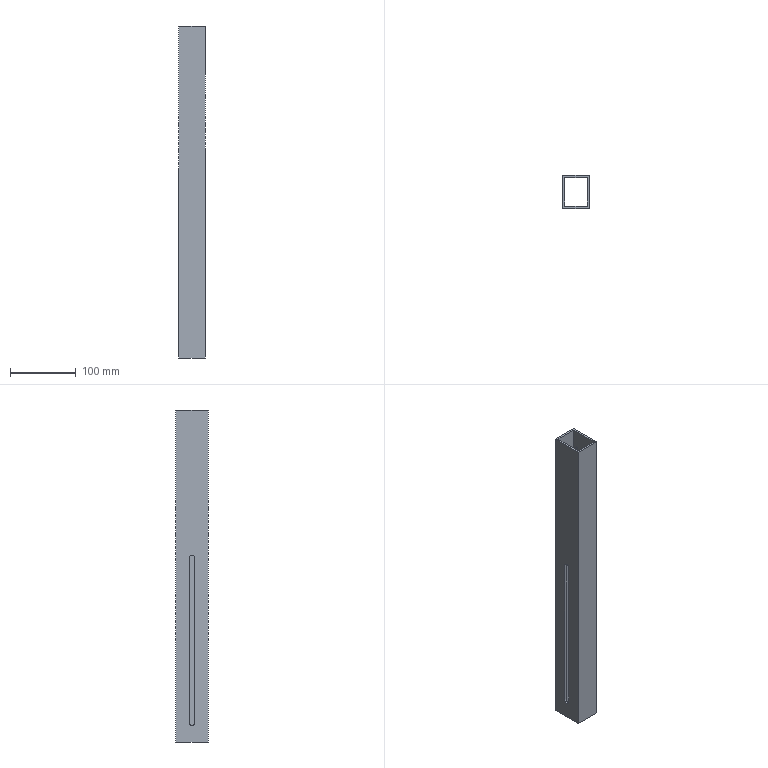Part | SolidWorks | features HoleWzd 4, ExtruThin 1 | 1 solid | 39 faces | box 40 x 50 x 506 mm | volume 247347 mm3 | cylinder 27 | plane 12 | commonest cylinder face diameters 5.5 x16 4.2 x8 9 x3
STEP:
#1=CARTESIAN_POINT('',(-17.,4.5,27.));
#2=VERTEX_POINT('',#1);
#3=CARTESIAN_POINT('',(-17.,0.,31.5));
#4=VERTEX_POINT('',#3);
#5=CARTESIAN_POINT('',(-17.,0.,27.));
#6=DIRECTION('',(1.,0.,0.));
#7=DIRECTION('',(0.,1.,0.));
#8=AXIS2_PLACEMENT_3D('',#5,#6,#7);
#9=CIRCLE('',#8,4.5);
#10=EDGE_CURVE('',#2,#4,#9,.T.);
#11=ORIENTED_EDGE('',*,*,#10,.T.);
#12=CARTESIAN_POINT('',(-20.,0.,31.5));
#13=VERTEX_POINT('',#12);
#14=CARTESIAN_POINT('',(-20.,0.,31.5));
#15=DIRECTION('',(-1.,0.,0.));
#16=VECTOR('',#15,1000.);
#17=LINE('',#14,#16);
#18=EDGE_CURVE('',#4,#13,#17,.T.);
#19=ORIENTED_EDGE('',*,*,#18,.T.);
#20=CARTESIAN_POINT('',(-20.,4.5,27.));
#21=VERTEX_POINT('',#20);
#22=CARTESIAN_POINT('',(-20.,0.,27.));
#23=DIRECTION('',(-1.,0.,0.));
#24=DIRECTION('',(0.,0.,1.));
#25=AXIS2_PLACEMENT_3D('',#22,#23,#24);
#26=CIRCLE('',#25,4.5);
#27=EDGE_CURVE('',#13,#21,#26,.T.);
#28=ORIENTED_EDGE('',*,*,#27,.T.);
#29=CARTESIAN_POINT('',(-16.999,4.5,27.));
#30=DIRECTION('',(1.,0.,0.));
#31=VECTOR('',#30,1000.);
#32=LINE('',#29,#31);
#33=EDGE_CURVE('',#21,#2,#32,.T.);
#34=ORIENTED_EDGE('',*,*,#33,.T.);
#35=EDGE_LOOP('',(#11,#19,#28,#34));
#36=FACE_OUTER_BOUND('',#35,.T.);
#37=CARTESIAN_POINT('',(-20.,0.,27.));
#38=DIRECTION('',(-1.,0.,0.));
#39=DIRECTION('',(0.,0.,1.));
#40=AXIS2_PLACEMENT_3D('',#37,#38,#39);
#41=CYLINDRICAL_SURFACE('',#40,4.5);
#42=ADVANCED_FACE('',(#36),#41,.F.);
#43=CARTESIAN_POINT('',(17.,15.,220.9));
#44=VERTEX_POINT('',#43);
#45=CARTESIAN_POINT('',(17.,15.,225.1));
#46=VERTEX_POINT('',#45);
#47=CARTESIAN_POINT('',(17.,15.,223.));
#48=DIRECTION('',(-1.,0.,0.));
#49=DIRECTION('',(0.,-1.,0.));
#50=AXIS2_PLACEMENT_3D('',#47,#48,#49);
#51=CIRCLE('',#50,2.1);
#52=EDGE_CURVE('',#44,#46,#51,.T.);
#53=ORIENTED_EDGE('',*,*,#52,.T.);
#54=CARTESIAN_POINT('',(20.,15.,225.1));
#55=VERTEX_POINT('',#54);
#56=CARTESIAN_POINT('',(20.,15.,225.1));
#57=DIRECTION('',(1.,0.,0.));
#58=VECTOR('',#57,1000.);
#59=LINE('',#56,#58);
#60=EDGE_CURVE('',#46,#55,#59,.T.);
#61=ORIENTED_EDGE('',*,*,#60,.T.);
#62=CARTESIAN_POINT('',(20.,15.,220.9));
#63=VERTEX_POINT('',#62);
#64=CARTESIAN_POINT('',(20.,15.,223.));
#65=DIRECTION('',(1.,0.,0.));
#66=DIRECTION('',(0.,0.,-1.));
#67=AXIS2_PLACEMENT_3D('',#64,#65,#66);
#68=CIRCLE('',#67,2.1);
#69=EDGE_CURVE('',#55,#63,#68,.T.);
#70=ORIENTED_EDGE('',*,*,#69,.T.);
#71=CARTESIAN_POINT('',(20.,15.,220.9));
#72=DIRECTION('',(1.,0.,0.));
#73=VECTOR('',#72,1000.);
#74=LINE('',#71,#73);
#75=EDGE_CURVE('',#44,#63,#74,.T.);
#76=ORIENTED_EDGE('',*,*,#75,.F.);
#77=EDGE_LOOP('',(#53,#61,#70,#76));
#78=FACE_OUTER_BOUND('',#77,.T.);
#79=CARTESIAN_POINT('',(20.,15.,223.));
#80=DIRECTION('',(1.,0.,0.));
#81=DIRECTION('',(0.,0.,-1.));
#82=AXIS2_PLACEMENT_3D('',#79,#80,#81);
#83=CYLINDRICAL_SURFACE('',#82,2.1);
#84=ADVANCED_FACE('',(#78),#83,.F.);
#85=CARTESIAN_POINT('',(17.,-15.,220.9));
#86=VERTEX_POINT('',#85);
#87=CARTESIAN_POINT('',(17.,-15.,225.1));
#88=VERTEX_POINT('',#87);
#89=CARTESIAN_POINT('',(17.,-15.,223.));
#90=DIRECTION('',(-1.,0.,0.));
#91=DIRECTION('',(0.,-1.,0.));
#92=AXIS2_PLACEMENT_3D('',#89,#90,#91);
#93=CIRCLE('',#92,2.1);
#94=EDGE_CURVE('',#86,#88,#93,.T.);
#95=ORIENTED_EDGE('',*,*,#94,.T.);
#96=CARTESIAN_POINT('',(20.,-15.,225.1));
#97=VERTEX_POINT('',#96);
#98=CARTESIAN_POINT('',(20.,-15.,225.1));
#99=DIRECTION('',(1.,0.,0.));
#100=VECTOR('',#99,1000.);
#101=LINE('',#98,#100);
#102=EDGE_CURVE('',#88,#97,#101,.T.);
#103=ORIENTED_EDGE('',*,*,#102,.T.);
#104=CARTESIAN_POINT('',(20.,-15.,220.9));
#105=VERTEX_POINT('',#104);
#106=CARTESIAN_POINT('',(20.,-15.,223.));
#107=DIRECTION('',(1.,0.,0.));
#108=DIRECTION('',(0.,0.,-1.));
#109=AXIS2_PLACEMENT_3D('',#106,#107,#108);
#110=CIRCLE('',#109,2.1);
#111=EDGE_CURVE('',#97,#105,#110,.T.);
#112=ORIENTED_EDGE('',*,*,#111,.T.);
#113=CARTESIAN_POINT('',(20.,-15.,220.9));
#114=DIRECTION('',(1.,0.,0.));
#115=VECTOR('',#114,1000.);
#116=LINE('',#113,#115);
#117=EDGE_CURVE('',#86,#105,#116,.T.);
#118=ORIENTED_EDGE('',*,*,#117,.F.);
#119=EDGE_LOOP('',(#95,#103,#112,#118));
#120=FACE_OUTER_BOUND('',#119,.T.);
#121=CARTESIAN_POINT('',(20.,-15.,223.));
#122=DIRECTION('',(1.,0.,0.));
#123=DIRECTION('',(0.,0.,-1.));
#124=AXIS2_PLACEMENT_3D('',#121,#122,#123);
#125=CYLINDRICAL_SURFACE('',#124,2.1);
#126=ADVANCED_FACE('',(#120),#125,.F.);
#127=CARTESIAN_POINT('',(17.,-15.,-225.1));
#128=VERTEX_POINT('',#127);
#129=CARTESIAN_POINT('',(17.,-15.,-220.9));
#130=VERTEX_POINT('',#129);
#131=CARTESIAN_POINT('',(17.,-15.,-223.));
#132=DIRECTION('',(-1.,0.,0.));
#133=DIRECTION('',(0.,-1.,0.));
#134=AXIS2_PLACEMENT_3D('',#131,#132,#133);
#135=CIRCLE('',#134,2.1);
#136=EDGE_CURVE('',#128,#130,#135,.T.);
#137=ORIENTED_EDGE('',*,*,#136,.T.);
#138=CARTESIAN_POINT('',(20.,-15.,-220.9));
#139=VERTEX_POINT('',#138);
#140=CARTESIAN_POINT('',(20.,-15.,-220.9));
#141=DIRECTION('',(1.,0.,0.));
#142=VECTOR('',#141,1000.);
#143=LINE('',#140,#142);
#144=EDGE_CURVE('',#130,#139,#143,.T.);
#145=ORIENTED_EDGE('',*,*,#144,.T.);
#146=CARTESIAN_POINT('',(20.,-15.,-225.1));
#147=VERTEX_POINT('',#146);
#148=CARTESIAN_POINT('',(20.,-15.,-223.));
#149=DIRECTION('',(1.,0.,0.));
#150=DIRECTION('',(0.,0.,-1.));
#151=AXIS2_PLACEMENT_3D('',#148,#149,#150);
#152=CIRCLE('',#151,2.1);
#153=EDGE_CURVE('',#139,#147,#152,.T.);
#154=ORIENTED_EDGE('',*,*,#153,.T.);
#155=CARTESIAN_POINT('',(20.,-15.,-225.1));
#156=DIRECTION('',(1.,0.,0.));
#157=VECTOR('',#156,1000.);
#158=LINE('',#155,#157);
#159=EDGE_CURVE('',#128,#147,#158,.T.);
#160=ORIENTED_EDGE('',*,*,#159,.F.);
#161=EDGE_LOOP('',(#137,#145,#154,#160));
#162=FACE_OUTER_BOUND('',#161,.T.);
#163=CARTESIAN_POINT('',(20.,-15.,-223.));
#164=DIRECTION('',(1.,0.,0.));
#165=DIRECTION('',(0.,0.,-1.));
#166=AXIS2_PLACEMENT_3D('',#163,#164,#165);
#167=CYLINDRICAL_SURFACE('',#166,2.1);
#168=ADVANCED_FACE('',(#162),#167,.F.);
#169=CARTESIAN_POINT('',(17.,15.,-225.1));
#170=VERTEX_POINT('',#169);
#171=CARTESIAN_POINT('',(17.,15.,-220.9));
#172=VERTEX_POINT('',#171);
#173=CARTESIAN_POINT('',(17.,15.,-223.));
#174=DIRECTION('',(-1.,0.,0.));
#175=DIRECTION('',(0.,-1.,0.));
#176=AXIS2_PLACEMENT_3D('',#173,#174,#175);
#177=CIRCLE('',#176,2.1);
#178=EDGE_CURVE('',#170,#172,#177,.T.);
#179=ORIENTED_EDGE('',*,*,#178,.T.);
#180=CARTESIAN_POINT('',(20.,15.,-220.9));
#181=VERTEX_POINT('',#180);
#182=CARTESIAN_POINT('',(20.,15.,-220.9));
#183=DIRECTION('',(1.,0.,0.));
#184=VECTOR('',#183,1000.);
#185=LINE('',#182,#184);
#186=EDGE_CURVE('',#172,#181,#185,.T.);
#187=ORIENTED_EDGE('',*,*,#186,.T.);
#188=CARTESIAN_POINT('',(20.,15.,-225.1));
#189=VERTEX_POINT('',#188);
#190=CARTESIAN_POINT('',(20.,15.,-223.));
#191=DIRECTION('',(1.,0.,0.));
#192=DIRECTION('',(0.,0.,-1.));
#193=AXIS2_PLACEMENT_3D('',#190,#191,#192);
#194=CIRCLE('',#193,2.1);
#195=EDGE_CURVE('',#181,#189,#194,.T.);
#196=ORIENTED_EDGE('',*,*,#195,.T.);
#197=CARTESIAN_POINT('',(20.,15.,-225.1));
#198=DIRECTION('',(1.,0.,0.));
#199=VECTOR('',#198,1000.);
#200=LINE('',#197,#199);
#201=EDGE_CURVE('',#170,#189,#200,.T.);
#202=ORIENTED_EDGE('',*,*,#201,.F.);
#203=EDGE_LOOP('',(#179,#187,#196,#202));
#204=FACE_OUTER_BOUND('',#203,.T.);
#205=CARTESIAN_POINT('',(20.,15.,-223.));
#206=DIRECTION('',(1.,0.,0.));
#207=DIRECTION('',(0.,0.,-1.));
#208=AXIS2_PLACEMENT_3D('',#205,#206,#207);
#209=CYLINDRICAL_SURFACE('',#208,2.1);
#210=ADVANCED_FACE('',(#204),#209,.F.);
#211=CARTESIAN_POINT('',(17.,16.,179.5));
#212=VERTEX_POINT('',#211);
#213=CARTESIAN_POINT('',(17.,16.,185.));
#214=VERTEX_POINT('',#213);
#215=CARTESIAN_POINT('',(17.,16.,182.25));
#216=DIRECTION('',(-1.,0.,0.));
#217=DIRECTION('',(0.,-1.,0.));
#218=AXIS2_PLACEMENT_3D('',#215,#216,#217);
#219=CIRCLE('',#218,2.75);
#220=EDGE_CURVE('',#212,#214,#219,.T.);
#221=ORIENTED_EDGE('',*,*,#220,.T.);
#222=CARTESIAN_POINT('',(20.,16.,185.));
#223=VERTEX_POINT('',#222);
#224=CARTESIAN_POINT('',(20.,16.,185.));
#225=DIRECTION('',(1.,0.,0.));
#226=VECTOR('',#225,1000.);
#227=LINE('',#224,#226);
#228=EDGE_CURVE('',#214,#223,#227,.T.);
#229=ORIENTED_EDGE('',*,*,#228,.T.);
#230=CARTESIAN_POINT('',(20.,16.,179.5));
#231=VERTEX_POINT('',#230);
#232=CARTESIAN_POINT('',(20.,16.,182.25));
#233=DIRECTION('',(1.,0.,0.));
#234=DIRECTION('',(0.,0.,-1.));
#235=AXIS2_PLACEMENT_3D('',#232,#233,#234);
#236=CIRCLE('',#235,2.75);
#237=EDGE_CURVE('',#223,#231,#236,.T.);
#238=ORIENTED_EDGE('',*,*,#237,.T.);
#239=CARTESIAN_POINT('',(20.,16.,179.5));
#240=DIRECTION('',(1.,0.,0.));
#241=VECTOR('',#240,1000.);
#242=LINE('',#239,#241);
#243=EDGE_CURVE('',#212,#231,#242,.T.);
#244=ORIENTED_EDGE('',*,*,#243,.F.);
#245=EDGE_LOOP('',(#221,#229,#238,#244));
#246=FACE_OUTER_BOUND('',#245,.T.);
#247=CARTESIAN_POINT('',(20.,16.,182.25));
#248=DIRECTION('',(1.,0.,0.));
#249=DIRECTION('',(0.,0.,-1.));
#250=AXIS2_PLACEMENT_3D('',#247,#248,#249);
#251=CYLINDRICAL_SURFACE('',#250,2.75);
#252=ADVANCED_FACE('',(#246),#251,.F.);
#253=CARTESIAN_POINT('',(17.,16.,143.5));
#254=VERTEX_POINT('',#253);
#255=CARTESIAN_POINT('',(17.,16.,149.));
#256=VERTEX_POINT('',#255);
#257=CARTESIAN_POINT('',(17.,16.,146.25));
#258=DIRECTION('',(-1.,0.,0.));
#259=DIRECTION('',(0.,-1.,0.));
#260=AXIS2_PLACEMENT_3D('',#257,#258,#259);
#261=CIRCLE('',#260,2.75);
#262=EDGE_CURVE('',#254,#256,#261,.T.);
#263=ORIENTED_EDGE('',*,*,#262,.T.);
#264=CARTESIAN_POINT('',(20.,16.,149.));
#265=VERTEX_POINT('',#264);
#266=CARTESIAN_POINT('',(20.,16.,149.));
#267=DIRECTION('',(1.,0.,0.));
#268=VECTOR('',#267,1000.);
#269=LINE('',#266,#268);
#270=EDGE_CURVE('',#256,#265,#269,.T.);
#271=ORIENTED_EDGE('',*,*,#270,.T.);
#272=CARTESIAN_POINT('',(20.,16.,143.5));
#273=VERTEX_POINT('',#272);
#274=CARTESIAN_POINT('',(20.,16.,146.25));
#275=DIRECTION('',(1.,0.,0.));
#276=DIRECTION('',(0.,0.,-1.));
#277=AXIS2_PLACEMENT_3D('',#274,#275,#276);
#278=CIRCLE('',#277,2.75);
#279=EDGE_CURVE('',#265,#273,#278,.T.);
#280=ORIENTED_EDGE('',*,*,#279,.T.);
#281=CARTESIAN_POINT('',(20.,16.,143.5));
#282=DIRECTION('',(1.,0.,0.));
#283=VECTOR('',#282,1000.);
#284=LINE('',#281,#283);
#285=EDGE_CURVE('',#254,#273,#284,.T.);
#286=ORIENTED_EDGE('',*,*,#285,.F.);
#287=EDGE_LOOP('',(#263,#271,#280,#286));
#288=FACE_OUTER_BOUND('',#287,.T.);
#289=CARTESIAN_POINT('',(20.,16.,146.25));
#290=DIRECTION('',(1.,0.,0.));
#291=DIRECTION('',(0.,0.,-1.));
#292=AXIS2_PLACEMENT_3D('',#289,#290,#291);
#293=CYLINDRICAL_SURFACE('',#292,2.75);
#294=ADVANCED_FACE('',(#288),#293,.F.);
#295=CARTESIAN_POINT('',(17.,16.,92.));
#296=VERTEX_POINT('',#295);
#297=CARTESIAN_POINT('',(17.,16.,97.5));
#298=VERTEX_POINT('',#297);
#299=CARTESIAN_POINT('',(17.,16.,94.75));
#300=DIRECTION('',(-1.,0.,0.));
#301=DIRECTION('',(0.,-1.,0.));
#302=AXIS2_PLACEMENT_3D('',#299,#300,#301);
#303=CIRCLE('',#302,2.75);
#304=EDGE_CURVE('',#296,#298,#303,.T.);
#305=ORIENTED_EDGE('',*,*,#304,.T.);
#306=CARTESIAN_POINT('',(20.,16.,97.5));
#307=VERTEX_POINT('',#306);
#308=CARTESIAN_POINT('',(20.,16.,97.5));
#309=DIRECTION('',(1.,0.,0.));
#310=VECTOR('',#309,1000.);
#311=LINE('',#308,#310);
#312=EDGE_CURVE('',#298,#307,#311,.T.);
#313=ORIENTED_EDGE('',*,*,#312,.T.);
#314=CARTESIAN_POINT('',(20.,16.,92.));
#315=VERTEX_POINT('',#314);
#316=CARTESIAN_POINT('',(20.,16.,94.75));
#317=DIRECTION('',(1.,0.,0.));
#318=DIRECTION('',(0.,0.,-1.));
#319=AXIS2_PLACEMENT_3D('',#316,#317,#318);
#320=CIRCLE('',#319,2.75);
#321=EDGE_CURVE('',#307,#315,#320,.T.);
#322=ORIENTED_EDGE('',*,*,#321,.T.);
#323=CARTESIAN_POINT('',(20.,16.,92.));
#324=DIRECTION('',(1.,0.,0.));
#325=VECTOR('',#324,1000.);
#326=LINE('',#323,#325);
#327=EDGE_CURVE('',#296,#315,#326,.T.);
#328=ORIENTED_EDGE('',*,*,#327,.F.);
#329=EDGE_LOOP('',(#305,#313,#322,#328));
#330=FACE_OUTER_BOUND('',#329,.T.);
#331=CARTESIAN_POINT('',(20.,16.,94.75));
#332=DIRECTION('',(1.,0.,0.));
#333=DIRECTION('',(0.,0.,-1.));
#334=AXIS2_PLACEMENT_3D('',#331,#332,#333);
#335=CYLINDRICAL_SURFACE('',#334,2.75);
#336=ADVANCED_FACE('',(#330),#335,.F.);
#337=CARTESIAN_POINT('',(17.,16.,56.));
#338=VERTEX_POINT('',#337);
#339=CARTESIAN_POINT('',(17.,16.,61.5));
#340=VERTEX_POINT('',#339);
#341=CARTESIAN_POINT('',(17.,16.,58.75));
#342=DIRECTION('',(-1.,0.,0.));
#343=DIRECTION('',(0.,-1.,0.));
#344=AXIS2_PLACEMENT_3D('',#341,#342,#343);
#345=CIRCLE('',#344,2.75);
#346=EDGE_CURVE('',#338,#340,#345,.T.);
#347=ORIENTED_EDGE('',*,*,#346,.T.);
#348=CARTESIAN_POINT('',(20.,16.,61.5));
#349=VERTEX_POINT('',#348);
#350=CARTESIAN_POINT('',(20.,16.,61.5));
#351=DIRECTION('',(1.,0.,0.));
#352=VECTOR('',#351,1000.);
#353=LINE('',#350,#352);
#354=EDGE_CURVE('',#340,#349,#353,.T.);
#355=ORIENTED_EDGE('',*,*,#354,.T.);
#356=CARTESIAN_POINT('',(20.,16.,56.));
#357=VERTEX_POINT('',#356);
#358=CARTESIAN_POINT('',(20.,16.,58.75));
#359=DIRECTION('',(1.,0.,0.));
#360=DIRECTION('',(0.,0.,-1.));
#361=AXIS2_PLACEMENT_3D('',#358,#359,#360);
#362=CIRCLE('',#361,2.75);
#363=EDGE_CURVE('',#349,#357,#362,.T.);
#364=ORIENTED_EDGE('',*,*,#363,.T.);
#365=CARTESIAN_POINT('',(20.,16.,56.));
#366=DIRECTION('',(1.,0.,0.));
#367=VECTOR('',#366,1000.);
#368=LINE('',#365,#367);
#369=EDGE_CURVE('',#338,#357,#368,.T.);
#370=ORIENTED_EDGE('',*,*,#369,.F.);
#371=EDGE_LOOP('',(#347,#355,#364,#370));
#372=FACE_OUTER_BOUND('',#371,.T.);
#373=CARTESIAN_POINT('',(20.,16.,58.75));
#374=DIRECTION('',(1.,0.,0.));
#375=DIRECTION('',(0.,0.,-1.));
#376=AXIS2_PLACEMENT_3D('',#373,#374,#375);
#377=CYLINDRICAL_SURFACE('',#376,2.75);
#378=ADVANCED_FACE('',(#372),#377,.F.);
#379=CARTESIAN_POINT('',(17.,-16.,56.));
#380=VERTEX_POINT('',#379);
#381=CARTESIAN_POINT('',(17.,-16.,61.5));
#382=VERTEX_POINT('',#381);
#383=CARTESIAN_POINT('',(17.,-16.,58.75));
#384=DIRECTION('',(-1.,0.,0.));
#385=DIRECTION('',(0.,-1.,0.));
#386=AXIS2_PLACEMENT_3D('',#383,#384,#385);
#387=CIRCLE('',#386,2.75);
#388=EDGE_CURVE('',#380,#382,#387,.T.);
#389=ORIENTED_EDGE('',*,*,#388,.T.);
#390=CARTESIAN_POINT('',(20.,-16.,61.5));
#391=VERTEX_POINT('',#390);
#392=CARTESIAN_POINT('',(20.,-16.,61.5));
#393=DIRECTION('',(1.,0.,0.));
#394=VECTOR('',#393,1000.);
#395=LINE('',#392,#394);
#396=EDGE_CURVE('',#382,#391,#395,.T.);
#397=ORIENTED_EDGE('',*,*,#396,.T.);
#398=CARTESIAN_POINT('',(20.,-16.,56.));
#399=VERTEX_POINT('',#398);
#400=CARTESIAN_POINT('',(20.,-16.,58.75));
#401=DIRECTION('',(1.,0.,0.));
#402=DIRECTION('',(0.,0.,-1.));
#403=AXIS2_PLACEMENT_3D('',#400,#401,#402);
#404=CIRCLE('',#403,2.75);
#405=EDGE_CURVE('',#391,#399,#404,.T.);
#406=ORIENTED_EDGE('',*,*,#405,.T.);
#407=CARTESIAN_POINT('',(20.,-16.,56.));
#408=DIRECTION('',(1.,0.,0.));
#409=VECTOR('',#408,1000.);
#410=LINE('',#407,#409);
#411=EDGE_CURVE('',#380,#399,#410,.T.);
#412=ORIENTED_EDGE('',*,*,#411,.F.);
#413=EDGE_LOOP('',(#389,#397,#406,#412));
#414=FACE_OUTER_BOUND('',#413,.T.);
#415=CARTESIAN_POINT('',(20.,-16.,58.75));
#416=DIRECTION('',(1.,0.,0.));
#417=DIRECTION('',(0.,0.,-1.));
#418=AXIS2_PLACEMENT_3D('',#415,#416,#417);
#419=CYLINDRICAL_SURFACE('',#418,2.75);
#420=ADVANCED_FACE('',(#414),#419,.F.);
#421=CARTESIAN_POINT('',(17.,-16.,92.));
#422=VERTEX_POINT('',#421);
#423=CARTESIAN_POINT('',(17.,-16.,97.5));
#424=VERTEX_POINT('',#423);
#425=CARTESIAN_POINT('',(17.,-16.,94.75));
#426=DIRECTION('',(-1.,0.,0.));
#427=DIRECTION('',(0.,-1.,0.));
#428=AXIS2_PLACEMENT_3D('',#425,#426,#427);
#429=CIRCLE('',#428,2.75);
#430=EDGE_CURVE('',#422,#424,#429,.T.);
#431=ORIENTED_EDGE('',*,*,#430,.T.);
#432=CARTESIAN_POINT('',(20.,-16.,97.5));
#433=VERTEX_POINT('',#432);
#434=CARTESIAN_POINT('',(20.,-16.,97.5));
#435=DIRECTION('',(1.,0.,0.));
#436=VECTOR('',#435,1000.);
#437=LINE('',#434,#436);
#438=EDGE_CURVE('',#424,#433,#437,.T.);
#439=ORIENTED_EDGE('',*,*,#438,.T.);
#440=CARTESIAN_POINT('',(20.,-16.,92.));
#441=VERTEX_POINT('',#440);
#442=CARTESIAN_POINT('',(20.,-16.,94.75));
#443=DIRECTION('',(1.,0.,0.));
#444=DIRECTION('',(0.,0.,-1.));
#445=AXIS2_PLACEMENT_3D('',#442,#443,#444);
#446=CIRCLE('',#445,2.75);
#447=EDGE_CURVE('',#433,#441,#446,.T.);
#448=ORIENTED_EDGE('',*,*,#447,.T.);
#449=CARTESIAN_POINT('',(20.,-16.,92.));
#450=DIRECTION('',(1.,0.,0.));
#451=VECTOR('',#450,1000.);
#452=LINE('',#449,#451);
#453=EDGE_CURVE('',#422,#441,#452,.T.);
#454=ORIENTED_EDGE('',*,*,#453,.F.);
#455=EDGE_LOOP('',(#431,#439,#448,#454));
#456=FACE_OUTER_BOUND('',#455,.T.);
#457=CARTESIAN_POINT('',(20.,-16.,94.75));
#458=DIRECTION('',(1.,0.,0.));
#459=DIRECTION('',(0.,0.,-1.));
#460=AXIS2_PLACEMENT_3D('',#457,#458,#459);
#461=CYLINDRICAL_SURFACE('',#460,2.75);
#462=ADVANCED_FACE('',(#456),#461,.F.);
#463=CARTESIAN_POINT('',(17.,-16.,143.5));
#464=VERTEX_POINT('',#463);
#465=CARTESIAN_POINT('',(17.,-16.,149.));
#466=VERTEX_POINT('',#465);
#467=CARTESIAN_POINT('',(17.,-16.,146.25));
#468=DIRECTION('',(-1.,0.,0.));
#469=DIRECTION('',(0.,-1.,0.));
#470=AXIS2_PLACEMENT_3D('',#467,#468,#469);
#471=CIRCLE('',#470,2.75);
#472=EDGE_CURVE('',#464,#466,#471,.T.);
#473=ORIENTED_EDGE('',*,*,#472,.T.);
#474=CARTESIAN_POINT('',(20.,-16.,149.));
#475=VERTEX_POINT('',#474);
#476=CARTESIAN_POINT('',(20.,-16.,149.));
#477=DIRECTION('',(1.,0.,0.));
#478=VECTOR('',#477,1000.);
#479=LINE('',#476,#478);
#480=EDGE_CURVE('',#466,#475,#479,.T.);
#481=ORIENTED_EDGE('',*,*,#480,.T.);
#482=CARTESIAN_POINT('',(20.,-16.,143.5));
#483=VERTEX_POINT('',#482);
#484=CARTESIAN_POINT('',(20.,-16.,146.25));
#485=DIRECTION('',(1.,0.,0.));
#486=DIRECTION('',(0.,0.,-1.));
#487=AXIS2_PLACEMENT_3D('',#484,#485,#486);
#488=CIRCLE('',#487,2.75);
#489=EDGE_CURVE('',#475,#483,#488,.T.);
#490=ORIENTED_EDGE('',*,*,#489,.T.);
#491=CARTESIAN_POINT('',(20.,-16.,143.5));
#492=DIRECTION('',(1.,0.,0.));
#493=VECTOR('',#492,1000.);
#494=LINE('',#491,#493);
#495=EDGE_CURVE('',#464,#483,#494,.T.);
#496=ORIENTED_EDGE('',*,*,#495,.F.);
#497=EDGE_LOOP('',(#473,#481,#490,#496));
#498=FACE_OUTER_BOUND('',#497,.T.);
#499=CARTESIAN_POINT('',(20.,-16.,146.25));
#500=DIRECTION('',(1.,0.,0.));
#501=DIRECTION('',(0.,0.,-1.));
#502=AXIS2_PLACEMENT_3D('',#499,#500,#501);
#503=CYLINDRICAL_SURFACE('',#502,2.75);
#504=ADVANCED_FACE('',(#498),#503,.F.);
#505=CARTESIAN_POINT('',(17.,-16.,179.5));
#506=VERTEX_POINT('',#505);
#507=CARTESIAN_POINT('',(17.,-16.,185.));
#508=VERTEX_POINT('',#507);
#509=CARTESIAN_POINT('',(17.,-16.,182.25));
#510=DIRECTION('',(-1.,0.,0.));
#511=DIRECTION('',(0.,-1.,0.));
#512=AXIS2_PLACEMENT_3D('',#509,#510,#511);
#513=CIRCLE('',#512,2.75);
#514=EDGE_CURVE('',#506,#508,#513,.T.);
#515=ORIENTED_EDGE('',*,*,#514,.T.);
#516=CARTESIAN_POINT('',(20.,-16.,185.));
#517=VERTEX_POINT('',#516);
#518=CARTESIAN_POINT('',(20.,-16.,185.));
#519=DIRECTION('',(1.,0.,0.));
#520=VECTOR('',#519,1000.);
#521=LINE('',#518,#520);
#522=EDGE_CURVE('',#508,#517,#521,.T.);
#523=ORIENTED_EDGE('',*,*,#522,.T.);
#524=CARTESIAN_POINT('',(20.,-16.,179.5));
#525=VERTEX_POINT('',#524);
#526=CARTESIAN_POINT('',(20.,-16.,182.25));
#527=DIRECTION('',(1.,0.,0.));
#528=DIRECTION('',(0.,0.,-1.));
#529=AXIS2_PLACEMENT_3D('',#526,#527,#528);
#530=CIRCLE('',#529,2.75);
#531=EDGE_CURVE('',#517,#525,#530,.T.);
#532=ORIENTED_EDGE('',*,*,#531,.T.);
#533=CARTESIAN_POINT('',(20.,-16.,179.5));
#534=DIRECTION('',(1.,0.,0.));
#535=VECTOR('',#534,1000.);
#536=LINE('',#533,#535);
#537=EDGE_CURVE('',#506,#525,#536,.T.);
#538=ORIENTED_EDGE('',*,*,#537,.F.);
#539=EDGE_LOOP('',(#515,#523,#532,#538));
#540=FACE_OUTER_BOUND('',#539,.T.);
#541=CARTESIAN_POINT('',(20.,-16.,182.25));
#542=DIRECTION('',(1.,0.,0.));
#543=DIRECTION('',(0.,0.,-1.));
#544=AXIS2_PLACEMENT_3D('',#541,#542,#543);
#545=CYLINDRICAL_SURFACE('',#544,2.75);
#546=ADVANCED_FACE('',(#540),#545,.F.);
#547=CARTESIAN_POINT('',(-20.,25.,-253.));
#548=VERTEX_POINT('',#547);
#549=CARTESIAN_POINT('',(-20.,-25.,-253.));
#550=VERTEX_POINT('',#549);
#551=CARTESIAN_POINT('',(-20.,25.,-253.));
#552=DIRECTION('',(0.,-1.,0.));
#553=VECTOR('',#552,1000.);
#554=LINE('',#551,#553);
#555=EDGE_CURVE('',#548,#550,#554,.T.);
#556=ORIENTED_EDGE('',*,*,#555,.T.);
#557=CARTESIAN_POINT('',(-20.,-25.,253.));
#558=VERTEX_POINT('',#557);
#559=CARTESIAN_POINT('',(-20.,-25.,253.));
#560=DIRECTION('',(0.,0.,-1.));
#561=VECTOR('',#560,1000.);
#562=LINE('',#559,#561);
#563=EDGE_CURVE('',#558,#550,#562,.T.);
#564=ORIENTED_EDGE('',*,*,#563,.F.);
#565=CARTESIAN_POINT('',(-20.,25.,253.));
#566=VERTEX_POINT('',#565);
#567=CARTESIAN_POINT('',(-20.,25.,253.));
#568=DIRECTION('',(0.,-1.,0.));
#569=VECTOR('',#568,1000.);
#570=LINE('',#567,#569);
#571=EDGE_CURVE('',#566,#558,#570,.T.);
#572=ORIENTED_EDGE('',*,*,#571,.F.);
#573=CARTESIAN_POINT('',(-20.,25.,253.));
#574=DIRECTION('',(0.,0.,-1.));
#575=VECTOR('',#574,1000.);
#576=LINE('',#573,#575);
#577=EDGE_CURVE('',#566,#548,#576,.T.);
#578=ORIENTED_EDGE('',*,*,#577,.T.);
#579=EDGE_LOOP('',(#556,#564,#572,#578));
#580=FACE_OUTER_BOUND('',#579,.T.);
#581=CARTESIAN_POINT('',(-20.,-4.5,-223.));
#582=VERTEX_POINT('',#581);
#583=CARTESIAN_POINT('',(-20.,-4.5,27.));
#584=VERTEX_POINT('',#583);
#585=CARTESIAN_POINT('',(-20.,-4.5,-223.));
#586=DIRECTION('',(0.,0.,1.));
#587=VECTOR('',#586,1000.);
#588=LINE('',#585,#587);
#589=EDGE_CURVE('',#582,#584,#588,.T.);
#590=ORIENTED_EDGE('',*,*,#589,.F.);
#591=CARTESIAN_POINT('',(-20.,4.5,-223.));
#592=VERTEX_POINT('',#591);
#593=CARTESIAN_POINT('',(-20.,0.,-223.));
#594=DIRECTION('',(-1.,0.,0.));
#595=DIRECTION('',(0.,0.,1.));
#596=AXIS2_PLACEMENT_3D('',#593,#594,#595);
#597=CIRCLE('',#596,4.5);
#598=EDGE_CURVE('',#592,#582,#597,.T.);
#599=ORIENTED_EDGE('',*,*,#598,.F.);
#600=CARTESIAN_POINT('',(-20.,4.5,-223.));
#601=DIRECTION('',(0.,0.,1.));
#602=VECTOR('',#601,1000.);
#603=LINE('',#600,#602);
#604=EDGE_CURVE('',#592,#21,#603,.T.);
#605=ORIENTED_EDGE('',*,*,#604,.T.);
#606=ORIENTED_EDGE('',*,*,#27,.F.);
#607=CARTESIAN_POINT('',(-20.,0.,27.));
#608=DIRECTION('',(-1.,0.,0.));
#609=DIRECTION('',(0.,0.,1.));
#610=AXIS2_PLACEMENT_3D('',#607,#608,#609);
#611=CIRCLE('',#610,4.5);
#612=EDGE_CURVE('',#584,#13,#611,.T.);
#613=ORIENTED_EDGE('',*,*,#612,.F.);
#614=EDGE_LOOP('',(#590,#599,#605,#606,#613));
#615=FACE_BOUND('',#614,.T.);
#616=CARTESIAN_POINT('',(-20.,25.,253.));
#617=DIRECTION('',(1.,0.,0.));
#618=DIRECTION('',(0.,1.,0.));
#619=AXIS2_PLACEMENT_3D('',#616,#617,#618);
#620=PLANE('',#619);
#621=ADVANCED_FACE('',(#580,#615),#620,.F.);
#622=CARTESIAN_POINT('',(-17.,22.,-253.));
#623=VERTEX_POINT('',#622);
#624=CARTESIAN_POINT('',(-17.,-22.,-253.));
#625=VERTEX_POINT('',#624);
#626=CARTESIAN_POINT('',(-17.,25.,-253.));
#627=DIRECTION('',(0.,-1.,0.));
#628=VECTOR('',#627,1000.);
#629=LINE('',#626,#628);
#630=EDGE_CURVE('',#623,#625,#629,.T.);
#631=ORIENTED_EDGE('',*,*,#630,.F.);
#632=CARTESIAN_POINT('',(-17.,22.,253.));
#633=VERTEX_POINT('',#632);
#634=CARTESIAN_POINT('',(-17.,22.,253.));
#635=DIRECTION('',(0.,0.,-1.));
#636=VECTOR('',#635,1000.);
#637=LINE('',#634,#636);
#638=EDGE_CURVE('',#633,#623,#637,.T.);
#639=ORIENTED_EDGE('',*,*,#638,.F.);
#640=CARTESIAN_POINT('',(-17.,-22.,253.));
#641=VERTEX_POINT('',#640);
#642=CARTESIAN_POINT('',(-17.,25.,253.));
#643=DIRECTION('',(0.,-1.,0.));
#644=VECTOR('',#643,1000.);
#645=LINE('',#642,#644);
#646=EDGE_CURVE('',#633,#641,#645,.T.);
#647=ORIENTED_EDGE('',*,*,#646,.T.);
#648=CARTESIAN_POINT('',(-17.,-22.,253.));
#649=DIRECTION('',(0.,0.,-1.));
#650=VECTOR('',#649,1000.);
#651=LINE('',#648,#650);
#652=EDGE_CURVE('',#641,#625,#651,.T.);
#653=ORIENTED_EDGE('',*,*,#652,.T.);
#654=EDGE_LOOP('',(#631,#639,#647,#653));
#655=FACE_OUTER_BOUND('',#654,.T.);
#656=ORIENTED_EDGE('',*,*,#10,.F.);
#657=CARTESIAN_POINT('',(-17.,4.5,-223.));
#658=VERTEX_POINT('',#657);
#659=CARTESIAN_POINT('',(-17.,4.5,253.));
#660=DIRECTION('',(0.,0.,-1.));
#661=VECTOR('',#660,1000.);
#662=LINE('',#659,#661);
#663=EDGE_CURVE('',#2,#658,#662,.T.);
#664=ORIENTED_EDGE('',*,*,#663,.T.);
#665=CARTESIAN_POINT('',(-17.,-4.5,-223.));
#666=VERTEX_POINT('',#665);
#667=CARTESIAN_POINT('',(-17.,0.,-223.));
#668=DIRECTION('',(1.,0.,0.));
#669=DIRECTION('',(0.,1.,0.));
#670=AXIS2_PLACEMENT_3D('',#667,#668,#669);
#671=CIRCLE('',#670,4.5);
#672=EDGE_CURVE('',#666,#658,#671,.T.);
#673=ORIENTED_EDGE('',*,*,#672,.F.);
#674=CARTESIAN_POINT('',(-17.,-4.5,27.));
#675=VERTEX_POINT('',#674);
#676=CARTESIAN_POINT('',(-17.,-4.5,253.));
#677=DIRECTION('',(0.,0.,-1.));
#678=VECTOR('',#677,1000.);
#679=LINE('',#676,#678);
#680=EDGE_CURVE('',#675,#666,#679,.T.);
#681=ORIENTED_EDGE('',*,*,#680,.F.);
#682=CARTESIAN_POINT('',(-17.,0.,27.));
#683=DIRECTION('',(1.,0.,0.));
#684=DIRECTION('',(0.,1.,0.));
#685=AXIS2_PLACEMENT_3D('',#682,#683,#684);
#686=CIRCLE('',#685,4.5);
#687=EDGE_CURVE('',#4,#675,#686,.T.);
#688=ORIENTED_EDGE('',*,*,#687,.F.);
#689=EDGE_LOOP('',(#656,#664,#673,#681,#688));
#690=FACE_BOUND('',#689,.T.);
#691=CARTESIAN_POINT('',(-17.,25.,253.));
#692=DIRECTION('',(1.,0.,0.));
#693=DIRECTION('',(0.,1.,0.));
#694=AXIS2_PLACEMENT_3D('',#691,#692,#693);
#695=PLANE('',#694);
#696=ADVANCED_FACE('',(#655,#690),#695,.T.);
#697=CARTESIAN_POINT('',(20.,-15.,223.));
#698=DIRECTION('',(1.,0.,0.));
#699=DIRECTION('',(0.,0.,-1.));
#700=AXIS2_PLACEMENT_3D('',#697,#698,#699);
#701=CIRCLE('',#700,2.1);
#702=EDGE_CURVE('',#105,#97,#701,.T.);
#703=ORIENTED_EDGE('',*,*,#702,.F.);
#704=ORIENTED_EDGE('',*,*,#111,.F.);
#705=EDGE_LOOP('',(#703,#704));
#706=FACE_BOUND('',#705,.T.);
#707=CARTESIAN_POINT('',(20.,-25.,-253.));
#708=VERTEX_POINT('',#707);
#709=CARTESIAN_POINT('',(20.,25.,-253.));
#710=VERTEX_POINT('',#709);
#711=CARTESIAN_POINT('',(20.,25.,-253.));
#712=DIRECTION('',(0.,1.,0.));
#713=VECTOR('',#712,1000.);
#714=LINE('',#711,#713);
#715=EDGE_CURVE('',#708,#710,#714,.T.);
#716=ORIENTED_EDGE('',*,*,#715,.T.);
#717=CARTESIAN_POINT('',(20.,25.,253.));
#718=VERTEX_POINT('',#717);
#719=CARTESIAN_POINT('',(20.,25.,253.));
#720=DIRECTION('',(0.,0.,-1.));
#721=VECTOR('',#720,1000.);
#722=LINE('',#719,#721);
#723=EDGE_CURVE('',#718,#710,#722,.T.);
#724=ORIENTED_EDGE('',*,*,#723,.F.);
#725=CARTESIAN_POINT('',(20.,-25.,253.));
#726=VERTEX_POINT('',#725);
#727=CARTESIAN_POINT('',(20.,25.,253.));
#728=DIRECTION('',(0.,1.,0.));
#729=VECTOR('',#728,1000.);
#730=LINE('',#727,#729);
#731=EDGE_CURVE('',#726,#718,#730,.T.);
#732=ORIENTED_EDGE('',*,*,#731,.F.);
#733=CARTESIAN_POINT('',(20.,-25.,253.));
#734=DIRECTION('',(0.,0.,-1.));
#735=VECTOR('',#734,1000.);
#736=LINE('',#733,#735);
#737=EDGE_CURVE('',#726,#708,#736,.T.);
#738=ORIENTED_EDGE('',*,*,#737,.T.);
#739=EDGE_LOOP('',(#716,#724,#732,#738));
#740=FACE_OUTER_BOUND('',#739,.T.);
#741=CARTESIAN_POINT('',(20.,-16.,182.25));
#742=DIRECTION('',(1.,0.,0.));
#743=DIRECTION('',(0.,0.,-1.));
#744=AXIS2_PLACEMENT_3D('',#741,#742,#743);
#745=CIRCLE('',#744,2.75);
#746=EDGE_CURVE('',#525,#517,#745,.T.);
#747=ORIENTED_EDGE('',*,*,#746,.F.);
#748=ORIENTED_EDGE('',*,*,#531,.F.);
#749=EDGE_LOOP('',(#747,#748));
#750=FACE_BOUND('',#749,.T.);
#751=CARTESIAN_POINT('',(20.,-16.,146.25));
#752=DIRECTION('',(1.,0.,0.));
#753=DIRECTION('',(0.,0.,-1.));
#754=AXIS2_PLACEMENT_3D('',#751,#752,#753);
#755=CIRCLE('',#754,2.75);
#756=EDGE_CURVE('',#483,#475,#755,.T.);
#757=ORIENTED_EDGE('',*,*,#756,.F.);
#758=ORIENTED_EDGE('',*,*,#489,.F.);
#759=EDGE_LOOP('',(#757,#758));
#760=FACE_BOUND('',#759,.T.);
#761=CARTESIAN_POINT('',(20.,-16.,94.75));
#762=DIRECTION('',(1.,0.,0.));
#763=DIRECTION('',(0.,0.,-1.));
#764=AXIS2_PLACEMENT_3D('',#761,#762,#763);
#765=CIRCLE('',#764,2.75);
#766=EDGE_CURVE('',#441,#433,#765,.T.);
#767=ORIENTED_EDGE('',*,*,#766,.F.);
#768=ORIENTED_EDGE('',*,*,#447,.F.);
#769=EDGE_LOOP('',(#767,#768));
#770=FACE_BOUND('',#769,.T.);
#771=CARTESIAN_POINT('',(20.,-16.,58.75));
#772=DIRECTION('',(1.,0.,0.));
#773=DIRECTION('',(0.,0.,-1.));
#774=AXIS2_PLACEMENT_3D('',#771,#772,#773);
#775=CIRCLE('',#774,2.75);
#776=EDGE_CURVE('',#399,#391,#775,.T.);
#777=ORIENTED_EDGE('',*,*,#776,.F.);
#778=ORIENTED_EDGE('',*,*,#405,.F.);
#779=EDGE_LOOP('',(#777,#778));
#780=FACE_BOUND('',#779,.T.);
#781=CARTESIAN_POINT('',(20.,16.,58.75));
#782=DIRECTION('',(1.,0.,0.));
#783=DIRECTION('',(0.,0.,-1.));
#784=AXIS2_PLACEMENT_3D('',#781,#782,#783);
#785=CIRCLE('',#784,2.75);
#786=EDGE_CURVE('',#357,#349,#785,.T.);
#787=ORIENTED_EDGE('',*,*,#786,.F.);
#788=ORIENTED_EDGE('',*,*,#363,.F.);
#789=EDGE_LOOP('',(#787,#788));
#790=FACE_BOUND('',#789,.T.);
#791=CARTESIAN_POINT('',(20.,16.,94.75));
#792=DIRECTION('',(1.,0.,0.));
#793=DIRECTION('',(0.,0.,-1.));
#794=AXIS2_PLACEMENT_3D('',#791,#792,#793);
#795=CIRCLE('',#794,2.75);
#796=EDGE_CURVE('',#315,#307,#795,.T.);
#797=ORIENTED_EDGE('',*,*,#796,.F.);
#798=ORIENTED_EDGE('',*,*,#321,.F.);
#799=EDGE_LOOP('',(#797,#798));
#800=FACE_BOUND('',#799,.T.);
#801=CARTESIAN_POINT('',(20.,16.,146.25));
#802=DIRECTION('',(1.,0.,0.));
#803=DIRECTION('',(0.,0.,-1.));
#804=AXIS2_PLACEMENT_3D('',#801,#802,#803);
#805=CIRCLE('',#804,2.75);
#806=EDGE_CURVE('',#273,#265,#805,.T.);
#807=ORIENTED_EDGE('',*,*,#806,.F.);
#808=ORIENTED_EDGE('',*,*,#279,.F.);
#809=EDGE_LOOP('',(#807,#808));
#810=FACE_BOUND('',#809,.T.);
#811=CARTESIAN_POINT('',(20.,16.,182.25));
#812=DIRECTION('',(1.,0.,0.));
#813=DIRECTION('',(0.,0.,-1.));
#814=AXIS2_PLACEMENT_3D('',#811,#812,#813);
#815=CIRCLE('',#814,2.75);
#816=EDGE_CURVE('',#231,#223,#815,.T.);
#817=ORIENTED_EDGE('',*,*,#816,.F.);
#818=ORIENTED_EDGE('',*,*,#237,.F.);
#819=EDGE_LOOP('',(#817,#818));
#820=FACE_BOUND('',#819,.T.);
#821=CARTESIAN_POINT('',(20.,15.,-223.));
#822=DIRECTION('',(1.,0.,0.));
#823=DIRECTION('',(0.,0.,-1.));
#824=AXIS2_PLACEMENT_3D('',#821,#822,#823);
#825=CIRCLE('',#824,2.1);
#826=EDGE_CURVE('',#189,#181,#825,.T.);
#827=ORIENTED_EDGE('',*,*,#826,.F.);
#828=ORIENTED_EDGE('',*,*,#195,.F.);
#829=EDGE_LOOP('',(#827,#828));
#830=FACE_BOUND('',#829,.T.);
#831=CARTESIAN_POINT('',(20.,-15.,-223.));
#832=DIRECTION('',(1.,0.,0.));
#833=DIRECTION('',(0.,0.,-1.));
#834=AXIS2_PLACEMENT_3D('',#831,#832,#833);
#835=CIRCLE('',#834,2.1);
#836=EDGE_CURVE('',#147,#139,#835,.T.);
#837=ORIENTED_EDGE('',*,*,#836,.F.);
#838=ORIENTED_EDGE('',*,*,#153,.F.);
#839=EDGE_LOOP('',(#837,#838));
#840=FACE_BOUND('',#839,.T.);
#841=CARTESIAN_POINT('',(20.,15.,223.));
#842=DIRECTION('',(1.,0.,0.));
#843=DIRECTION('',(0.,0.,-1.));
#844=AXIS2_PLACEMENT_3D('',#841,#842,#843);
#845=CIRCLE('',#844,2.1);
#846=EDGE_CURVE('',#63,#55,#845,.T.);
#847=ORIENTED_EDGE('',*,*,#846,.F.);
#848=ORIENTED_EDGE('',*,*,#69,.F.);
#849=EDGE_LOOP('',(#847,#848));
#850=FACE_BOUND('',#849,.T.);
#851=CARTESIAN_POINT('',(20.,25.,253.));
#852=DIRECTION('',(-1.,0.,0.));
#853=DIRECTION('',(0.,-1.,0.));
#854=AXIS2_PLACEMENT_3D('',#851,#852,#853);
#855=PLANE('',#854);
#856=ADVANCED_FACE('',(#706,#740,#750,#760,#770,#780,#790,#800,#810,#820,#830,#840,#850),#855,.F.);
#857=ORIENTED_EDGE('',*,*,#731,.T.);
#858=CARTESIAN_POINT('',(-20.,25.,253.));
#859=DIRECTION('',(-1.,0.,0.));
#860=VECTOR('',#859,1000.);
#861=LINE('',#858,#860);
#862=EDGE_CURVE('',#718,#566,#861,.T.);
#863=ORIENTED_EDGE('',*,*,#862,.T.);
#864=ORIENTED_EDGE('',*,*,#571,.T.);
#865=CARTESIAN_POINT('',(-20.,-25.,253.));
#866=DIRECTION('',(1.,0.,0.));
#867=VECTOR('',#866,1000.);
#868=LINE('',#865,#867);
#869=EDGE_CURVE('',#558,#726,#868,.T.);
#870=ORIENTED_EDGE('',*,*,#869,.T.);
#871=EDGE_LOOP('',(#857,#863,#864,#870));
#872=FACE_OUTER_BOUND('',#871,.T.);
#873=CARTESIAN_POINT('',(17.,22.,253.));
#874=VERTEX_POINT('',#873);
#875=CARTESIAN_POINT('',(-20.,22.,253.));
#876=DIRECTION('',(-1.,0.,0.));
#877=VECTOR('',#876,1000.);
#878=LINE('',#875,#877);
#879=EDGE_CURVE('',#874,#633,#878,.T.);
#880=ORIENTED_EDGE('',*,*,#879,.F.);
#881=CARTESIAN_POINT('',(17.,-22.,253.));
#882=VERTEX_POINT('',#881);
#883=CARTESIAN_POINT('',(17.,25.,253.));
#884=DIRECTION('',(0.,1.,0.));
#885=VECTOR('',#884,1000.);
#886=LINE('',#883,#885);
#887=EDGE_CURVE('',#882,#874,#886,.T.);
#888=ORIENTED_EDGE('',*,*,#887,.F.);
#889=CARTESIAN_POINT('',(-20.,-22.,253.));
#890=DIRECTION('',(1.,0.,0.));
#891=VECTOR('',#890,1000.);
#892=LINE('',#889,#891);
#893=EDGE_CURVE('',#641,#882,#892,.T.);
#894=ORIENTED_EDGE('',*,*,#893,.F.);
#895=ORIENTED_EDGE('',*,*,#646,.F.);
#896=EDGE_LOOP('',(#880,#888,#894,#895));
#897=FACE_BOUND('',#896,.T.);
#898=CARTESIAN_POINT('',(0.,0.,253.));
#899=DIRECTION('',(0.,0.,1.));
#900=DIRECTION('',(1.,0.,0.));
#901=AXIS2_PLACEMENT_3D('',#898,#899,#900);
#902=PLANE('',#901);
#903=ADVANCED_FACE('',(#872,#897),#902,.T.);
#904=ORIENTED_EDGE('',*,*,#715,.F.);
#905=CARTESIAN_POINT('',(-20.,-25.,-253.));
#906=DIRECTION('',(1.,0.,0.));
#907=VECTOR('',#906,1000.);
#908=LINE('',#905,#907);
#909=EDGE_CURVE('',#550,#708,#908,.T.);
#910=ORIENTED_EDGE('',*,*,#909,.F.);
#911=ORIENTED_EDGE('',*,*,#555,.F.);
#912=CARTESIAN_POINT('',(-20.,25.,-253.));
#913=DIRECTION('',(-1.,0.,0.));
#914=VECTOR('',#913,1000.);
#915=LINE('',#912,#914);
#916=EDGE_CURVE('',#710,#548,#915,.T.);
#917=ORIENTED_EDGE('',*,*,#916,.F.);
#918=EDGE_LOOP('',(#904,#910,#911,#917));
#919=FACE_OUTER_BOUND('',#918,.T.);
#920=CARTESIAN_POINT('',(17.,-22.,-253.));
#921=VERTEX_POINT('',#920);
#922=CARTESIAN_POINT('',(17.,22.,-253.));
#923=VERTEX_POINT('',#922);
#924=CARTESIAN_POINT('',(17.,25.,-253.));
#925=DIRECTION('',(0.,1.,0.));
#926=VECTOR('',#925,1000.);
#927=LINE('',#924,#926);
#928=EDGE_CURVE('',#921,#923,#927,.T.);
#929=ORIENTED_EDGE('',*,*,#928,.T.);
#930=CARTESIAN_POINT('',(-20.,22.,-253.));
#931=DIRECTION('',(-1.,0.,0.));
#932=VECTOR('',#931,1000.);
#933=LINE('',#930,#932);
#934=EDGE_CURVE('',#923,#623,#933,.T.);
#935=ORIENTED_EDGE('',*,*,#934,.T.);
#936=ORIENTED_EDGE('',*,*,#630,.T.);
#937=CARTESIAN_POINT('',(-20.,-22.,-253.));
#938=DIRECTION('',(1.,0.,0.));
#939=VECTOR('',#938,1000.);
#940=LINE('',#937,#939);
#941=EDGE_CURVE('',#625,#921,#940,.T.);
#942=ORIENTED_EDGE('',*,*,#941,.T.);
#943=EDGE_LOOP('',(#929,#935,#936,#942));
#944=FACE_BOUND('',#943,.T.);
#945=CARTESIAN_POINT('',(0.,0.,-253.));
#946=DIRECTION('',(0.,0.,1.));
#947=DIRECTION('',(1.,0.,0.));
#948=AXIS2_PLACEMENT_3D('',#945,#946,#947);
#949=PLANE('',#948);
#950=ADVANCED_FACE('',(#919,#944),#949,.F.);
#951=ORIENTED_EDGE('',*,*,#916,.T.);
#952=ORIENTED_EDGE('',*,*,#577,.F.);
#953=ORIENTED_EDGE('',*,*,#862,.F.);
#954=ORIENTED_EDGE('',*,*,#723,.T.);
#955=EDGE_LOOP('',(#951,#952,#953,#954));
#956=FACE_OUTER_BOUND('',#955,.T.);
#957=CARTESIAN_POINT('',(-20.,25.,253.));
#958=DIRECTION('',(0.,-1.,0.));
#959=DIRECTION('',(1.,0.,0.));
#960=AXIS2_PLACEMENT_3D('',#957,#958,#959);
#961=PLANE('',#960);
#962=ADVANCED_FACE('',(#956),#961,.F.);
#963=ORIENTED_EDGE('',*,*,#909,.T.);
#964=ORIENTED_EDGE('',*,*,#737,.F.);
#965=ORIENTED_EDGE('',*,*,#869,.F.);
#966=ORIENTED_EDGE('',*,*,#563,.T.);
#967=EDGE_LOOP('',(#963,#964,#965,#966));
#968=FACE_OUTER_BOUND('',#967,.T.);
#969=CARTESIAN_POINT('',(-20.,-25.,253.));
#970=DIRECTION('',(0.,1.,0.));
#971=DIRECTION('',(0.,0.,1.));
#972=AXIS2_PLACEMENT_3D('',#969,#970,#971);
#973=PLANE('',#972);
#974=ADVANCED_FACE('',(#968),#973,.F.);
#975=ORIENTED_EDGE('',*,*,#52,.F.);
#976=CARTESIAN_POINT('',(17.,15.,223.));
#977=DIRECTION('',(-1.,0.,0.));
#978=DIRECTION('',(0.,-1.,0.));
#979=AXIS2_PLACEMENT_3D('',#976,#977,#978);
#980=CIRCLE('',#979,2.1);
#981=EDGE_CURVE('',#46,#44,#980,.T.);
#982=ORIENTED_EDGE('',*,*,#981,.F.);
#983=EDGE_LOOP('',(#975,#982));
#984=FACE_BOUND('',#983,.T.);
#985=ORIENTED_EDGE('',*,*,#94,.F.);
#986=CARTESIAN_POINT('',(17.,-15.,223.));
#987=DIRECTION('',(-1.,0.,0.));
#988=DIRECTION('',(0.,-1.,0.));
#989=AXIS2_PLACEMENT_3D('',#986,#987,#988);
#990=CIRCLE('',#989,2.1);
#991=EDGE_CURVE('',#88,#86,#990,.T.);
#992=ORIENTED_EDGE('',*,*,#991,.F.);
#993=EDGE_LOOP('',(#985,#992));
#994=FACE_BOUND('',#993,.T.);
#995=ORIENTED_EDGE('',*,*,#136,.F.);
#996=CARTESIAN_POINT('',(17.,-15.,-223.));
#997=DIRECTION('',(-1.,0.,0.));
#998=DIRECTION('',(0.,-1.,0.));
#999=AXIS2_PLACEMENT_3D('',#996,#997,#998);
#1000=CIRCLE('',#999,2.1);
#1001=EDGE_CURVE('',#130,#128,#1000,.T.);
#1002=ORIENTED_EDGE('',*,*,#1001,.F.);
#1003=EDGE_LOOP('',(#995,#1002));
#1004=FACE_BOUND('',#1003,.T.);
#1005=ORIENTED_EDGE('',*,*,#178,.F.);
#1006=CARTESIAN_POINT('',(17.,15.,-223.));
#1007=DIRECTION('',(-1.,0.,0.));
#1008=DIRECTION('',(0.,-1.,0.));
#1009=AXIS2_PLACEMENT_3D('',#1006,#1007,#1008);
#1010=CIRCLE('',#1009,2.1);
#1011=EDGE_CURVE('',#172,#170,#1010,.T.);
#1012=ORIENTED_EDGE('',*,*,#1011,.F.);
#1013=EDGE_LOOP('',(#1005,#1012));
#1014=FACE_BOUND('',#1013,.T.);
#1015=ORIENTED_EDGE('',*,*,#220,.F.);
#1016=CARTESIAN_POINT('',(17.,16.,182.25));
#1017=DIRECTION('',(-1.,0.,0.));
#1018=DIRECTION('',(0.,-1.,0.));
#1019=AXIS2_PLACEMENT_3D('',#1016,#1017,#1018);
#1020=CIRCLE('',#1019,2.75);
#1021=EDGE_CURVE('',#214,#212,#1020,.T.);
#1022=ORIENTED_EDGE('',*,*,#1021,.F.);
#1023=EDGE_LOOP('',(#1015,#1022));
#1024=FACE_BOUND('',#1023,.T.);
#1025=ORIENTED_EDGE('',*,*,#262,.F.);
#1026=CARTESIAN_POINT('',(17.,16.,146.25));
#1027=DIRECTION('',(-1.,0.,0.));
#1028=DIRECTION('',(0.,-1.,0.));
#1029=AXIS2_PLACEMENT_3D('',#1026,#1027,#1028);
#1030=CIRCLE('',#1029,2.75);
#1031=EDGE_CURVE('',#256,#254,#1030,.T.);
#1032=ORIENTED_EDGE('',*,*,#1031,.F.);
#1033=EDGE_LOOP('',(#1025,#1032));
#1034=FACE_BOUND('',#1033,.T.);
#1035=ORIENTED_EDGE('',*,*,#304,.F.);
#1036=CARTESIAN_POINT('',(17.,16.,94.75));
#1037=DIRECTION('',(-1.,0.,0.));
#1038=DIRECTION('',(0.,-1.,0.));
#1039=AXIS2_PLACEMENT_3D('',#1036,#1037,#1038);
#1040=CIRCLE('',#1039,2.75);
#1041=EDGE_CURVE('',#298,#296,#1040,.T.);
#1042=ORIENTED_EDGE('',*,*,#1041,.F.);
#1043=EDGE_LOOP('',(#1035,#1042));
#1044=FACE_BOUND('',#1043,.T.);
#1045=ORIENTED_EDGE('',*,*,#346,.F.);
#1046=CARTESIAN_POINT('',(17.,16.,58.75));
#1047=DIRECTION('',(-1.,0.,0.));
#1048=DIRECTION('',(0.,-1.,0.));
#1049=AXIS2_PLACEMENT_3D('',#1046,#1047,#1048);
#1050=CIRCLE('',#1049,2.75);
#1051=EDGE_CURVE('',#340,#338,#1050,.T.);
#1052=ORIENTED_EDGE('',*,*,#1051,.F.);
#1053=EDGE_LOOP('',(#1045,#1052));
#1054=FACE_BOUND('',#1053,.T.);
#1055=ORIENTED_EDGE('',*,*,#388,.F.);
#1056=CARTESIAN_POINT('',(17.,-16.,58.75));
#1057=DIRECTION('',(-1.,0.,0.));
#1058=DIRECTION('',(0.,-1.,0.));
#1059=AXIS2_PLACEMENT_3D('',#1056,#1057,#1058);
#1060=CIRCLE('',#1059,2.75);
#1061=EDGE_CURVE('',#382,#380,#1060,.T.);
#1062=ORIENTED_EDGE('',*,*,#1061,.F.);
#1063=EDGE_LOOP('',(#1055,#1062));
#1064=FACE_BOUND('',#1063,.T.);
#1065=ORIENTED_EDGE('',*,*,#430,.F.);
#1066=CARTESIAN_POINT('',(17.,-16.,94.75));
#1067=DIRECTION('',(-1.,0.,0.));
#1068=DIRECTION('',(0.,-1.,0.));
#1069=AXIS2_PLACEMENT_3D('',#1066,#1067,#1068);
#1070=CIRCLE('',#1069,2.75);
#1071=EDGE_CURVE('',#424,#422,#1070,.T.);
#1072=ORIENTED_EDGE('',*,*,#1071,.F.);
#1073=EDGE_LOOP('',(#1065,#1072));
#1074=FACE_BOUND('',#1073,.T.);
#1075=ORIENTED_EDGE('',*,*,#472,.F.);
#1076=CARTESIAN_POINT('',(17.,-16.,146.25));
#1077=DIRECTION('',(-1.,0.,0.));
#1078=DIRECTION('',(0.,-1.,0.));
#1079=AXIS2_PLACEMENT_3D('',#1076,#1077,#1078);
#1080=CIRCLE('',#1079,2.75);
#1081=EDGE_CURVE('',#466,#464,#1080,.T.);
#1082=ORIENTED_EDGE('',*,*,#1081,.F.);
#1083=EDGE_LOOP('',(#1075,#1082));
#1084=FACE_BOUND('',#1083,.T.);
#1085=ORIENTED_EDGE('',*,*,#514,.F.);
#1086=CARTESIAN_POINT('',(17.,-16.,182.25));
#1087=DIRECTION('',(-1.,0.,0.));
#1088=DIRECTION('',(0.,-1.,0.));
#1089=AXIS2_PLACEMENT_3D('',#1086,#1087,#1088);
#1090=CIRCLE('',#1089,2.75);
#1091=EDGE_CURVE('',#508,#506,#1090,.T.);
#1092=ORIENTED_EDGE('',*,*,#1091,.F.);
#1093=EDGE_LOOP('',(#1085,#1092));
#1094=FACE_BOUND('',#1093,.T.);
#1095=ORIENTED_EDGE('',*,*,#928,.F.);
#1096=CARTESIAN_POINT('',(17.,-22.,253.));
#1097=DIRECTION('',(0.,0.,-1.));
#1098=VECTOR('',#1097,1000.);
#1099=LINE('',#1096,#1098);
#1100=EDGE_CURVE('',#882,#921,#1099,.T.);
#1101=ORIENTED_EDGE('',*,*,#1100,.F.);
#1102=ORIENTED_EDGE('',*,*,#887,.T.);
#1103=CARTESIAN_POINT('',(17.,22.,253.));
#1104=DIRECTION('',(0.,0.,-1.));
#1105=VECTOR('',#1104,1000.);
#1106=LINE('',#1103,#1105);
#1107=EDGE_CURVE('',#874,#923,#1106,.T.);
#1108=ORIENTED_EDGE('',*,*,#1107,.T.);
#1109=EDGE_LOOP('',(#1095,#1101,#1102,#1108));
#1110=FACE_OUTER_BOUND('',#1109,.T.);
#1111=CARTESIAN_POINT('',(17.,25.,253.));
#1112=DIRECTION('',(-1.,0.,0.));
#1113=DIRECTION('',(0.,-1.,0.));
#1114=AXIS2_PLACEMENT_3D('',#1111,#1112,#1113);
#1115=PLANE('',#1114);
#1116=ADVANCED_FACE('',(#984,#994,#1004,#1014,#1024,#1034,#1044,#1054,#1064,#1074,#1084,#1094,#1110),#1115,.T.);
#1117=ORIENTED_EDGE('',*,*,#934,.F.);
#1118=ORIENTED_EDGE('',*,*,#1107,.F.);
#1119=ORIENTED_EDGE('',*,*,#879,.T.);
#1120=ORIENTED_EDGE('',*,*,#638,.T.);
#1121=EDGE_LOOP('',(#1117,#1118,#1119,#1120));
#1122=FACE_OUTER_BOUND('',#1121,.T.);
#1123=CARTESIAN_POINT('',(-20.,22.,253.));
#1124=DIRECTION('',(0.,-1.,0.));
#1125=DIRECTION('',(1.,0.,0.));
#1126=AXIS2_PLACEMENT_3D('',#1123,#1124,#1125);
#1127=PLANE('',#1126);
#1128=ADVANCED_FACE('',(#1122),#1127,.T.);
#1129=ORIENTED_EDGE('',*,*,#941,.F.);
#1130=ORIENTED_EDGE('',*,*,#652,.F.);
#1131=ORIENTED_EDGE('',*,*,#893,.T.);
#1132=ORIENTED_EDGE('',*,*,#1100,.T.);
#1133=EDGE_LOOP('',(#1129,#1130,#1131,#1132));
#1134=FACE_OUTER_BOUND('',#1133,.T.);
#1135=CARTESIAN_POINT('',(-20.,-22.,253.));
#1136=DIRECTION('',(0.,1.,0.));
#1137=DIRECTION('',(0.,0.,1.));
#1138=AXIS2_PLACEMENT_3D('',#1135,#1136,#1137);
#1139=PLANE('',#1138);
#1140=ADVANCED_FACE('',(#1134),#1139,.T.);
#1141=ORIENTED_EDGE('',*,*,#522,.F.);
#1142=ORIENTED_EDGE('',*,*,#1091,.T.);
#1143=ORIENTED_EDGE('',*,*,#537,.T.);
#1144=ORIENTED_EDGE('',*,*,#746,.T.);
#1145=EDGE_LOOP('',(#1141,#1142,#1143,#1144));
#1146=FACE_OUTER_BOUND('',#1145,.T.);
#1147=CARTESIAN_POINT('',(20.,-16.,182.25));
#1148=DIRECTION('',(1.,0.,0.));
#1149=DIRECTION('',(0.,0.,-1.));
#1150=AXIS2_PLACEMENT_3D('',#1147,#1148,#1149);
#1151=CYLINDRICAL_SURFACE('',#1150,2.75);
#1152=ADVANCED_FACE('',(#1146),#1151,.F.);
#1153=ORIENTED_EDGE('',*,*,#480,.F.);
#1154=ORIENTED_EDGE('',*,*,#1081,.T.);
#1155=ORIENTED_EDGE('',*,*,#495,.T.);
#1156=ORIENTED_EDGE('',*,*,#756,.T.);
#1157=EDGE_LOOP('',(#1153,#1154,#1155,#1156));
#1158=FACE_OUTER_BOUND('',#1157,.T.);
#1159=CARTESIAN_POINT('',(20.,-16.,146.25));
#1160=DIRECTION('',(1.,0.,0.));
#1161=DIRECTION('',(0.,0.,-1.));
#1162=AXIS2_PLACEMENT_3D('',#1159,#1160,#1161);
#1163=CYLINDRICAL_SURFACE('',#1162,2.75);
#1164=ADVANCED_FACE('',(#1158),#1163,.F.);
#1165=ORIENTED_EDGE('',*,*,#438,.F.);
#1166=ORIENTED_EDGE('',*,*,#1071,.T.);
#1167=ORIENTED_EDGE('',*,*,#453,.T.);
#1168=ORIENTED_EDGE('',*,*,#766,.T.);
#1169=EDGE_LOOP('',(#1165,#1166,#1167,#1168));
#1170=FACE_OUTER_BOUND('',#1169,.T.);
#1171=CARTESIAN_POINT('',(20.,-16.,94.75));
#1172=DIRECTION('',(1.,0.,0.));
#1173=DIRECTION('',(0.,0.,-1.));
#1174=AXIS2_PLACEMENT_3D('',#1171,#1172,#1173);
#1175=CYLINDRICAL_SURFACE('',#1174,2.75);
#1176=ADVANCED_FACE('',(#1170),#1175,.F.);
#1177=ORIENTED_EDGE('',*,*,#396,.F.);
#1178=ORIENTED_EDGE('',*,*,#1061,.T.);
#1179=ORIENTED_EDGE('',*,*,#411,.T.);
#1180=ORIENTED_EDGE('',*,*,#776,.T.);
#1181=EDGE_LOOP('',(#1177,#1178,#1179,#1180));
#1182=FACE_OUTER_BOUND('',#1181,.T.);
#1183=CARTESIAN_POINT('',(20.,-16.,58.75));
#1184=DIRECTION('',(1.,0.,0.));
#1185=DIRECTION('',(0.,0.,-1.));
#1186=AXIS2_PLACEMENT_3D('',#1183,#1184,#1185);
#1187=CYLINDRICAL_SURFACE('',#1186,2.75);
#1188=ADVANCED_FACE('',(#1182),#1187,.F.);
#1189=ORIENTED_EDGE('',*,*,#354,.F.);
#1190=ORIENTED_EDGE('',*,*,#1051,.T.);
#1191=ORIENTED_EDGE('',*,*,#369,.T.);
#1192=ORIENTED_EDGE('',*,*,#786,.T.);
#1193=EDGE_LOOP('',(#1189,#1190,#1191,#1192));
#1194=FACE_OUTER_BOUND('',#1193,.T.);
#1195=CARTESIAN_POINT('',(20.,16.,58.75));
#1196=DIRECTION('',(1.,0.,0.));
#1197=DIRECTION('',(0.,0.,-1.));
#1198=AXIS2_PLACEMENT_3D('',#1195,#1196,#1197);
#1199=CYLINDRICAL_SURFACE('',#1198,2.75);
#1200=ADVANCED_FACE('',(#1194),#1199,.F.);
#1201=ORIENTED_EDGE('',*,*,#312,.F.);
#1202=ORIENTED_EDGE('',*,*,#1041,.T.);
#1203=ORIENTED_EDGE('',*,*,#327,.T.);
#1204=ORIENTED_EDGE('',*,*,#796,.T.);
#1205=EDGE_LOOP('',(#1201,#1202,#1203,#1204));
#1206=FACE_OUTER_BOUND('',#1205,.T.);
#1207=CARTESIAN_POINT('',(20.,16.,94.75));
#1208=DIRECTION('',(1.,0.,0.));
#1209=DIRECTION('',(0.,0.,-1.));
#1210=AXIS2_PLACEMENT_3D('',#1207,#1208,#1209);
#1211=CYLINDRICAL_SURFACE('',#1210,2.75);
#1212=ADVANCED_FACE('',(#1206),#1211,.F.);
#1213=ORIENTED_EDGE('',*,*,#270,.F.);
#1214=ORIENTED_EDGE('',*,*,#1031,.T.);
#1215=ORIENTED_EDGE('',*,*,#285,.T.);
#1216=ORIENTED_EDGE('',*,*,#806,.T.);
#1217=EDGE_LOOP('',(#1213,#1214,#1215,#1216));
#1218=FACE_OUTER_BOUND('',#1217,.T.);
#1219=CARTESIAN_POINT('',(20.,16.,146.25));
#1220=DIRECTION('',(1.,0.,0.));
#1221=DIRECTION('',(0.,0.,-1.));
#1222=AXIS2_PLACEMENT_3D('',#1219,#1220,#1221);
#1223=CYLINDRICAL_SURFACE('',#1222,2.75);
#1224=ADVANCED_FACE('',(#1218),#1223,.F.);
#1225=ORIENTED_EDGE('',*,*,#228,.F.);
#1226=ORIENTED_EDGE('',*,*,#1021,.T.);
#1227=ORIENTED_EDGE('',*,*,#243,.T.);
#1228=ORIENTED_EDGE('',*,*,#816,.T.);
#1229=EDGE_LOOP('',(#1225,#1226,#1227,#1228));
#1230=FACE_OUTER_BOUND('',#1229,.T.);
#1231=CARTESIAN_POINT('',(20.,16.,182.25));
#1232=DIRECTION('',(1.,0.,0.));
#1233=DIRECTION('',(0.,0.,-1.));
#1234=AXIS2_PLACEMENT_3D('',#1231,#1232,#1233);
#1235=CYLINDRICAL_SURFACE('',#1234,2.75);
#1236=ADVANCED_FACE('',(#1230),#1235,.F.);
#1237=ORIENTED_EDGE('',*,*,#186,.F.);
#1238=ORIENTED_EDGE('',*,*,#1011,.T.);
#1239=ORIENTED_EDGE('',*,*,#201,.T.);
#1240=ORIENTED_EDGE('',*,*,#826,.T.);
#1241=EDGE_LOOP('',(#1237,#1238,#1239,#1240));
#1242=FACE_OUTER_BOUND('',#1241,.T.);
#1243=CARTESIAN_POINT('',(20.,15.,-223.));
#1244=DIRECTION('',(1.,0.,0.));
#1245=DIRECTION('',(0.,0.,-1.));
#1246=AXIS2_PLACEMENT_3D('',#1243,#1244,#1245);
#1247=CYLINDRICAL_SURFACE('',#1246,2.1);
#1248=ADVANCED_FACE('',(#1242),#1247,.F.);
#1249=ORIENTED_EDGE('',*,*,#144,.F.);
#1250=ORIENTED_EDGE('',*,*,#1001,.T.);
#1251=ORIENTED_EDGE('',*,*,#159,.T.);
#1252=ORIENTED_EDGE('',*,*,#836,.T.);
#1253=EDGE_LOOP('',(#1249,#1250,#1251,#1252));
#1254=FACE_OUTER_BOUND('',#1253,.T.);
#1255=CARTESIAN_POINT('',(20.,-15.,-223.));
#1256=DIRECTION('',(1.,0.,0.));
#1257=DIRECTION('',(0.,0.,-1.));
#1258=AXIS2_PLACEMENT_3D('',#1255,#1256,#1257);
#1259=CYLINDRICAL_SURFACE('',#1258,2.1);
#1260=ADVANCED_FACE('',(#1254),#1259,.F.);
#1261=ORIENTED_EDGE('',*,*,#102,.F.);
#1262=ORIENTED_EDGE('',*,*,#991,.T.);
#1263=ORIENTED_EDGE('',*,*,#117,.T.);
#1264=ORIENTED_EDGE('',*,*,#702,.T.);
#1265=EDGE_LOOP('',(#1261,#1262,#1263,#1264));
#1266=FACE_OUTER_BOUND('',#1265,.T.);
#1267=CARTESIAN_POINT('',(20.,-15.,223.));
#1268=DIRECTION('',(1.,0.,0.));
#1269=DIRECTION('',(0.,0.,-1.));
#1270=AXIS2_PLACEMENT_3D('',#1267,#1268,#1269);
#1271=CYLINDRICAL_SURFACE('',#1270,2.1);
#1272=ADVANCED_FACE('',(#1266),#1271,.F.);
#1273=ORIENTED_EDGE('',*,*,#60,.F.);
#1274=ORIENTED_EDGE('',*,*,#981,.T.);
#1275=ORIENTED_EDGE('',*,*,#75,.T.);
#1276=ORIENTED_EDGE('',*,*,#846,.T.);
#1277=EDGE_LOOP('',(#1273,#1274,#1275,#1276));
#1278=FACE_OUTER_BOUND('',#1277,.T.);
#1279=CARTESIAN_POINT('',(20.,15.,223.));
#1280=DIRECTION('',(1.,0.,0.));
#1281=DIRECTION('',(0.,0.,-1.));
#1282=AXIS2_PLACEMENT_3D('',#1279,#1280,#1281);
#1283=CYLINDRICAL_SURFACE('',#1282,2.1);
#1284=ADVANCED_FACE('',(#1278),#1283,.F.);
#1285=ORIENTED_EDGE('',*,*,#18,.F.);
#1286=ORIENTED_EDGE('',*,*,#687,.T.);
#1287=CARTESIAN_POINT('',(-20.,-4.5,27.));
#1288=DIRECTION('',(1.,0.,0.));
#1289=VECTOR('',#1288,1000.);
#1290=LINE('',#1287,#1289);
#1291=EDGE_CURVE('',#584,#675,#1290,.T.);
#1292=ORIENTED_EDGE('',*,*,#1291,.F.);
#1293=ORIENTED_EDGE('',*,*,#612,.T.);
#1294=EDGE_LOOP('',(#1285,#1286,#1292,#1293));
#1295=FACE_OUTER_BOUND('',#1294,.T.);
#1296=CARTESIAN_POINT('',(-20.,0.,27.));
#1297=DIRECTION('',(-1.,0.,0.));
#1298=DIRECTION('',(0.,0.,1.));
#1299=AXIS2_PLACEMENT_3D('',#1296,#1297,#1298);
#1300=CYLINDRICAL_SURFACE('',#1299,4.5);
#1301=ADVANCED_FACE('',(#1295),#1300,.F.);
#1302=ORIENTED_EDGE('',*,*,#672,.T.);
#1303=CARTESIAN_POINT('',(-16.999,4.5,-223.));
#1304=DIRECTION('',(1.,0.,0.));
#1305=VECTOR('',#1304,1000.);
#1306=LINE('',#1303,#1305);
#1307=EDGE_CURVE('',#592,#658,#1306,.T.);
#1308=ORIENTED_EDGE('',*,*,#1307,.F.);
#1309=ORIENTED_EDGE('',*,*,#598,.T.);
#1310=CARTESIAN_POINT('',(-20.,-4.5,-223.));
#1311=DIRECTION('',(-1.,0.,0.));
#1312=VECTOR('',#1311,1000.);
#1313=LINE('',#1310,#1312);
#1314=EDGE_CURVE('',#666,#582,#1313,.T.);
#1315=ORIENTED_EDGE('',*,*,#1314,.F.);
#1316=EDGE_LOOP('',(#1302,#1308,#1309,#1315));
#1317=FACE_OUTER_BOUND('',#1316,.T.);
#1318=CARTESIAN_POINT('',(-20.,0.,-223.));
#1319=DIRECTION('',(-1.,0.,0.));
#1320=DIRECTION('',(0.,0.,1.));
#1321=AXIS2_PLACEMENT_3D('',#1318,#1319,#1320);
#1322=CYLINDRICAL_SURFACE('',#1321,4.5);
#1323=ADVANCED_FACE('',(#1317),#1322,.F.);
#1324=ORIENTED_EDGE('',*,*,#33,.F.);
#1325=ORIENTED_EDGE('',*,*,#604,.F.);
#1326=ORIENTED_EDGE('',*,*,#1307,.T.);
#1327=ORIENTED_EDGE('',*,*,#663,.F.);
#1328=EDGE_LOOP('',(#1324,#1325,#1326,#1327));
#1329=FACE_OUTER_BOUND('',#1328,.T.);
#1330=CARTESIAN_POINT('',(-16.999,4.5,-223.));
#1331=DIRECTION('',(0.,-1.,0.));
#1332=DIRECTION('',(1.,0.,0.));
#1333=AXIS2_PLACEMENT_3D('',#1330,#1331,#1332);
#1334=PLANE('',#1333);
#1335=ADVANCED_FACE('',(#1329),#1334,.T.);
#1336=ORIENTED_EDGE('',*,*,#680,.T.);
#1337=ORIENTED_EDGE('',*,*,#1314,.T.);
#1338=ORIENTED_EDGE('',*,*,#589,.T.);
#1339=ORIENTED_EDGE('',*,*,#1291,.T.);
#1340=EDGE_LOOP('',(#1336,#1337,#1338,#1339));
#1341=FACE_OUTER_BOUND('',#1340,.T.);
#1342=CARTESIAN_POINT('',(-20.,-4.5,-223.));
#1343=DIRECTION('',(0.,-1.,0.));
#1344=DIRECTION('',(0.,0.,-1.));
#1345=AXIS2_PLACEMENT_3D('',#1342,#1343,#1344);
#1346=PLANE('',#1345);
#1347=ADVANCED_FACE('',(#1341),#1346,.F.);
#1348=CLOSED_SHELL('',(#42,#84,#126,#168,#210,#252,#294,#336,#378,#420,#462,#504,#546,#621,#696,#856,#903,#950,#962,#974,#1116,#1128,#1140,#1152,#1164,#1176,#1188,#1200,#1212,#1224,#1236,#1248,#1260,#1272,#1284,#1301,#1323,#1335,#1347));
#1349=MANIFOLD_SOLID_BREP('',#1348);
#1350=CARTESIAN_POINT('',(0.,0.,0.));
#1351=DIRECTION('',(0.,0.,1.));
#1352=DIRECTION('',(1.,0.,0.));
#1353=AXIS2_PLACEMENT_3D('',#1350,#1351,#1352);
#1354=(LENGTH_UNIT()NAMED_UNIT(*)SI_UNIT(.MILLI.,.METRE.));
#1355=UNCERTAINTY_MEASURE_WITH_UNIT(LENGTH_MEASURE(0.00001),#1354,'','');
#1356=(NAMED_UNIT(*)PLANE_ANGLE_UNIT()SI_UNIT($,.RADIAN.));
#1357=(NAMED_UNIT(*)SI_UNIT($,.STERADIAN.)SOLID_ANGLE_UNIT());
#1358=(GEOMETRIC_REPRESENTATION_CONTEXT(3)GLOBAL_UNCERTAINTY_ASSIGNED_CONTEXT((#1355))GLOBAL_UNIT_ASSIGNED_CONTEXT((#1354,#1356,#1357))REPRESENTATION_CONTEXT('',''));
#1359=ADVANCED_BREP_SHAPE_REPRESENTATION('',(#1349,#1353),#1358);